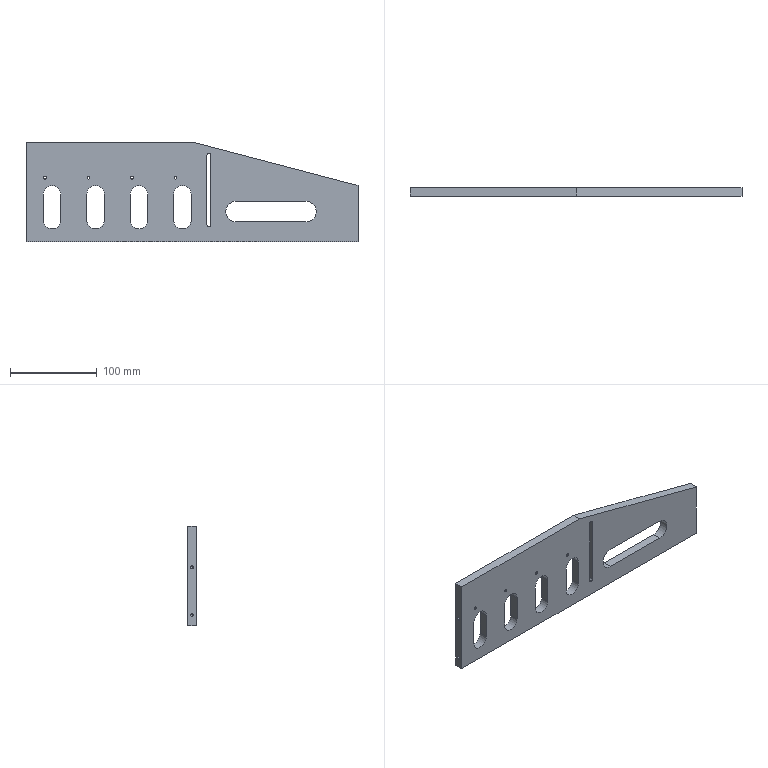Part | SolidWorks | features HoleWzd 4, ICE 3, LPattern 2, Chamfer 1, Cut 1, Extrusion 1, MoveFace 1 | 1 solid | 60 faces | box 382 x 10 x 115 mm | volume 327144 mm3 | cylinder 33 | plane 19 | cone 8 | commonest cylinder face diameters 3.3 x12 20 x12 2.5 x4 4.5 x3 24 x2